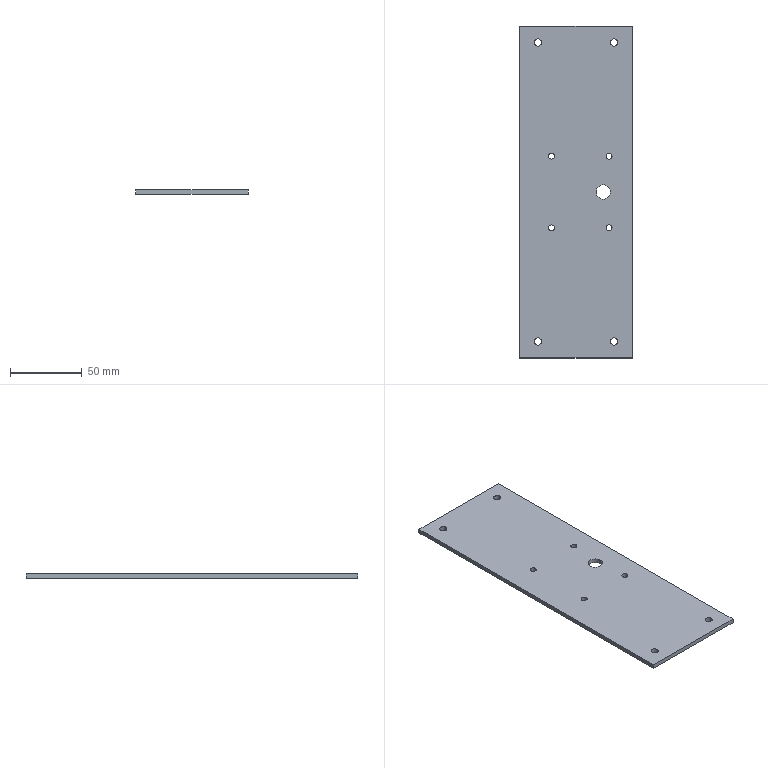Part | SolidWorks | features BaseBody 1 | 1 solid | 24 faces | box 78 x 231 x 3 mm | volume 53417 mm3 | cylinder 18 | plane 6 | commonest cylinder face diameters 4.2 x8 5 x8 10 x2
STEP:
#1=CARTESIAN_POINT('',(-19.1,-25.,3.));
#2=VERTEX_POINT('',#1);
#3=CARTESIAN_POINT('',(-14.9,-25.,3.));
#4=VERTEX_POINT('',#3);
#5=CARTESIAN_POINT('',(-17.,-25.,3.));
#6=DIRECTION('',(0.,0.,1.));
#7=DIRECTION('',(-1.,0.,0.));
#8=AXIS2_PLACEMENT_3D('',#5,#6,#7);
#9=CIRCLE('',#8,2.1);
#10=EDGE_CURVE('',#2,#4,#9,.T.);
#11=ORIENTED_EDGE('',*,*,#10,.T.);
#12=CARTESIAN_POINT('',(-14.9,-25.,0.));
#13=VERTEX_POINT('',#12);
#14=CARTESIAN_POINT('',(-14.9,-25.,3.));
#15=DIRECTION('',(0.,0.,-1.));
#16=VECTOR('',#15,1000.);
#17=LINE('',#14,#16);
#18=EDGE_CURVE('',#4,#13,#17,.T.);
#19=ORIENTED_EDGE('',*,*,#18,.T.);
#20=CARTESIAN_POINT('',(-19.1,-25.,0.));
#21=VERTEX_POINT('',#20);
#22=CARTESIAN_POINT('',(-17.,-25.,0.));
#23=DIRECTION('',(0.,0.,1.));
#24=DIRECTION('',(-1.,0.,0.));
#25=AXIS2_PLACEMENT_3D('',#22,#23,#24);
#26=CIRCLE('',#25,2.1);
#27=EDGE_CURVE('',#21,#13,#26,.T.);
#28=ORIENTED_EDGE('',*,*,#27,.F.);
#29=CARTESIAN_POINT('',(-19.1,-25.,3.));
#30=DIRECTION('',(0.,0.,-1.));
#31=VECTOR('',#30,1000.);
#32=LINE('',#29,#31);
#33=EDGE_CURVE('',#2,#21,#32,.T.);
#34=ORIENTED_EDGE('',*,*,#33,.F.);
#35=EDGE_LOOP('',(#11,#19,#28,#34));
#36=FACE_OUTER_BOUND('',#35,.T.);
#37=CARTESIAN_POINT('',(-17.,-25.,3.));
#38=DIRECTION('',(0.,0.,-1.));
#39=DIRECTION('',(-1.,0.,0.));
#40=AXIS2_PLACEMENT_3D('',#37,#38,#39);
#41=CYLINDRICAL_SURFACE('',#40,2.1);
#42=ADVANCED_FACE('',(#36),#41,.F.);
#43=CARTESIAN_POINT('',(20.9,-25.,3.));
#44=VERTEX_POINT('',#43);
#45=CARTESIAN_POINT('',(25.1,-25.,3.));
#46=VERTEX_POINT('',#45);
#47=CARTESIAN_POINT('',(23.,-25.,3.));
#48=DIRECTION('',(0.,0.,1.));
#49=DIRECTION('',(-1.,0.,0.));
#50=AXIS2_PLACEMENT_3D('',#47,#48,#49);
#51=CIRCLE('',#50,2.1);
#52=EDGE_CURVE('',#44,#46,#51,.T.);
#53=ORIENTED_EDGE('',*,*,#52,.T.);
#54=CARTESIAN_POINT('',(25.1,-25.,0.));
#55=VERTEX_POINT('',#54);
#56=CARTESIAN_POINT('',(25.1,-25.,3.));
#57=DIRECTION('',(0.,0.,-1.));
#58=VECTOR('',#57,1000.);
#59=LINE('',#56,#58);
#60=EDGE_CURVE('',#46,#55,#59,.T.);
#61=ORIENTED_EDGE('',*,*,#60,.T.);
#62=CARTESIAN_POINT('',(20.9,-25.,0.));
#63=VERTEX_POINT('',#62);
#64=CARTESIAN_POINT('',(23.,-25.,0.));
#65=DIRECTION('',(0.,0.,1.));
#66=DIRECTION('',(-1.,0.,0.));
#67=AXIS2_PLACEMENT_3D('',#64,#65,#66);
#68=CIRCLE('',#67,2.1);
#69=EDGE_CURVE('',#63,#55,#68,.T.);
#70=ORIENTED_EDGE('',*,*,#69,.F.);
#71=CARTESIAN_POINT('',(20.9,-25.,3.));
#72=DIRECTION('',(0.,0.,-1.));
#73=VECTOR('',#72,1000.);
#74=LINE('',#71,#73);
#75=EDGE_CURVE('',#44,#63,#74,.T.);
#76=ORIENTED_EDGE('',*,*,#75,.F.);
#77=EDGE_LOOP('',(#53,#61,#70,#76));
#78=FACE_OUTER_BOUND('',#77,.T.);
#79=CARTESIAN_POINT('',(23.,-25.,3.));
#80=DIRECTION('',(0.,0.,-1.));
#81=DIRECTION('',(-1.,0.,0.));
#82=AXIS2_PLACEMENT_3D('',#79,#80,#81);
#83=CYLINDRICAL_SURFACE('',#82,2.1);
#84=ADVANCED_FACE('',(#78),#83,.F.);
#85=CARTESIAN_POINT('',(20.9,25.,3.));
#86=VERTEX_POINT('',#85);
#87=CARTESIAN_POINT('',(25.1,25.,3.));
#88=VERTEX_POINT('',#87);
#89=CARTESIAN_POINT('',(23.,25.,3.));
#90=DIRECTION('',(0.,0.,1.));
#91=DIRECTION('',(-1.,0.,0.));
#92=AXIS2_PLACEMENT_3D('',#89,#90,#91);
#93=CIRCLE('',#92,2.1);
#94=EDGE_CURVE('',#86,#88,#93,.T.);
#95=ORIENTED_EDGE('',*,*,#94,.T.);
#96=CARTESIAN_POINT('',(25.1,25.,0.));
#97=VERTEX_POINT('',#96);
#98=CARTESIAN_POINT('',(25.1,25.,3.));
#99=DIRECTION('',(0.,0.,-1.));
#100=VECTOR('',#99,1000.);
#101=LINE('',#98,#100);
#102=EDGE_CURVE('',#88,#97,#101,.T.);
#103=ORIENTED_EDGE('',*,*,#102,.T.);
#104=CARTESIAN_POINT('',(20.9,25.,0.));
#105=VERTEX_POINT('',#104);
#106=CARTESIAN_POINT('',(23.,25.,0.));
#107=DIRECTION('',(0.,0.,1.));
#108=DIRECTION('',(-1.,0.,0.));
#109=AXIS2_PLACEMENT_3D('',#106,#107,#108);
#110=CIRCLE('',#109,2.1);
#111=EDGE_CURVE('',#105,#97,#110,.T.);
#112=ORIENTED_EDGE('',*,*,#111,.F.);
#113=CARTESIAN_POINT('',(20.9,25.,3.));
#114=DIRECTION('',(0.,0.,-1.));
#115=VECTOR('',#114,1000.);
#116=LINE('',#113,#115);
#117=EDGE_CURVE('',#86,#105,#116,.T.);
#118=ORIENTED_EDGE('',*,*,#117,.F.);
#119=EDGE_LOOP('',(#95,#103,#112,#118));
#120=FACE_OUTER_BOUND('',#119,.T.);
#121=CARTESIAN_POINT('',(23.,25.,3.));
#122=DIRECTION('',(0.,0.,-1.));
#123=DIRECTION('',(-1.,0.,0.));
#124=AXIS2_PLACEMENT_3D('',#121,#122,#123);
#125=CYLINDRICAL_SURFACE('',#124,2.1);
#126=ADVANCED_FACE('',(#120),#125,.F.);
#127=CARTESIAN_POINT('',(14.,0.,3.));
#128=VERTEX_POINT('',#127);
#129=CARTESIAN_POINT('',(24.,0.,3.));
#130=VERTEX_POINT('',#129);
#131=CARTESIAN_POINT('',(19.,0.,3.));
#132=DIRECTION('',(0.,0.,1.));
#133=DIRECTION('',(-1.,0.,0.));
#134=AXIS2_PLACEMENT_3D('',#131,#132,#133);
#135=CIRCLE('',#134,5.);
#136=EDGE_CURVE('',#128,#130,#135,.T.);
#137=ORIENTED_EDGE('',*,*,#136,.T.);
#138=CARTESIAN_POINT('',(24.,0.,0.));
#139=VERTEX_POINT('',#138);
#140=CARTESIAN_POINT('',(24.,0.,3.));
#141=DIRECTION('',(0.,0.,-1.));
#142=VECTOR('',#141,1000.);
#143=LINE('',#140,#142);
#144=EDGE_CURVE('',#130,#139,#143,.T.);
#145=ORIENTED_EDGE('',*,*,#144,.T.);
#146=CARTESIAN_POINT('',(14.,0.,0.));
#147=VERTEX_POINT('',#146);
#148=CARTESIAN_POINT('',(19.,0.,0.));
#149=DIRECTION('',(0.,0.,1.));
#150=DIRECTION('',(-1.,0.,0.));
#151=AXIS2_PLACEMENT_3D('',#148,#149,#150);
#152=CIRCLE('',#151,5.);
#153=EDGE_CURVE('',#147,#139,#152,.T.);
#154=ORIENTED_EDGE('',*,*,#153,.F.);
#155=CARTESIAN_POINT('',(14.,0.,3.));
#156=DIRECTION('',(0.,0.,-1.));
#157=VECTOR('',#156,1000.);
#158=LINE('',#155,#157);
#159=EDGE_CURVE('',#128,#147,#158,.T.);
#160=ORIENTED_EDGE('',*,*,#159,.F.);
#161=EDGE_LOOP('',(#137,#145,#154,#160));
#162=FACE_OUTER_BOUND('',#161,.T.);
#163=CARTESIAN_POINT('',(19.,0.,3.));
#164=DIRECTION('',(0.,0.,-1.));
#165=DIRECTION('',(-1.,0.,0.));
#166=AXIS2_PLACEMENT_3D('',#163,#164,#165);
#167=CYLINDRICAL_SURFACE('',#166,5.);
#168=ADVANCED_FACE('',(#162),#167,.F.);
#169=CARTESIAN_POINT('',(-29.,-104.,3.));
#170=VERTEX_POINT('',#169);
#171=CARTESIAN_POINT('',(-24.,-104.,3.));
#172=VERTEX_POINT('',#171);
#173=CARTESIAN_POINT('',(-26.5,-104.,3.));
#174=DIRECTION('',(0.,0.,1.));
#175=DIRECTION('',(-1.,0.,0.));
#176=AXIS2_PLACEMENT_3D('',#173,#174,#175);
#177=CIRCLE('',#176,2.5);
#178=EDGE_CURVE('',#170,#172,#177,.T.);
#179=ORIENTED_EDGE('',*,*,#178,.T.);
#180=CARTESIAN_POINT('',(-24.,-104.,0.));
#181=VERTEX_POINT('',#180);
#182=CARTESIAN_POINT('',(-24.,-104.,3.));
#183=DIRECTION('',(0.,0.,-1.));
#184=VECTOR('',#183,1000.);
#185=LINE('',#182,#184);
#186=EDGE_CURVE('',#172,#181,#185,.T.);
#187=ORIENTED_EDGE('',*,*,#186,.T.);
#188=CARTESIAN_POINT('',(-29.,-104.,0.));
#189=VERTEX_POINT('',#188);
#190=CARTESIAN_POINT('',(-26.5,-104.,0.));
#191=DIRECTION('',(0.,0.,1.));
#192=DIRECTION('',(-1.,0.,0.));
#193=AXIS2_PLACEMENT_3D('',#190,#191,#192);
#194=CIRCLE('',#193,2.5);
#195=EDGE_CURVE('',#189,#181,#194,.T.);
#196=ORIENTED_EDGE('',*,*,#195,.F.);
#197=CARTESIAN_POINT('',(-29.,-104.,3.));
#198=DIRECTION('',(0.,0.,-1.));
#199=VECTOR('',#198,1000.);
#200=LINE('',#197,#199);
#201=EDGE_CURVE('',#170,#189,#200,.T.);
#202=ORIENTED_EDGE('',*,*,#201,.F.);
#203=EDGE_LOOP('',(#179,#187,#196,#202));
#204=FACE_OUTER_BOUND('',#203,.T.);
#205=CARTESIAN_POINT('',(-26.5,-104.,3.));
#206=DIRECTION('',(0.,0.,-1.));
#207=DIRECTION('',(-1.,0.,0.));
#208=AXIS2_PLACEMENT_3D('',#205,#206,#207);
#209=CYLINDRICAL_SURFACE('',#208,2.5);
#210=ADVANCED_FACE('',(#204),#209,.F.);
#211=CARTESIAN_POINT('',(24.,-104.,3.));
#212=VERTEX_POINT('',#211);
#213=CARTESIAN_POINT('',(29.,-104.,3.));
#214=VERTEX_POINT('',#213);
#215=CARTESIAN_POINT('',(26.5,-104.,3.));
#216=DIRECTION('',(0.,0.,1.));
#217=DIRECTION('',(-1.,0.,0.));
#218=AXIS2_PLACEMENT_3D('',#215,#216,#217);
#219=CIRCLE('',#218,2.5);
#220=EDGE_CURVE('',#212,#214,#219,.T.);
#221=ORIENTED_EDGE('',*,*,#220,.T.);
#222=CARTESIAN_POINT('',(29.,-104.,0.));
#223=VERTEX_POINT('',#222);
#224=CARTESIAN_POINT('',(29.,-104.,3.));
#225=DIRECTION('',(0.,0.,-1.));
#226=VECTOR('',#225,1000.);
#227=LINE('',#224,#226);
#228=EDGE_CURVE('',#214,#223,#227,.T.);
#229=ORIENTED_EDGE('',*,*,#228,.T.);
#230=CARTESIAN_POINT('',(24.,-104.,0.));
#231=VERTEX_POINT('',#230);
#232=CARTESIAN_POINT('',(26.5,-104.,0.));
#233=DIRECTION('',(0.,0.,1.));
#234=DIRECTION('',(-1.,0.,0.));
#235=AXIS2_PLACEMENT_3D('',#232,#233,#234);
#236=CIRCLE('',#235,2.5);
#237=EDGE_CURVE('',#231,#223,#236,.T.);
#238=ORIENTED_EDGE('',*,*,#237,.F.);
#239=CARTESIAN_POINT('',(24.,-104.,3.));
#240=DIRECTION('',(0.,0.,-1.));
#241=VECTOR('',#240,1000.);
#242=LINE('',#239,#241);
#243=EDGE_CURVE('',#212,#231,#242,.T.);
#244=ORIENTED_EDGE('',*,*,#243,.F.);
#245=EDGE_LOOP('',(#221,#229,#238,#244));
#246=FACE_OUTER_BOUND('',#245,.T.);
#247=CARTESIAN_POINT('',(26.5,-104.,3.));
#248=DIRECTION('',(0.,0.,-1.));
#249=DIRECTION('',(-1.,0.,0.));
#250=AXIS2_PLACEMENT_3D('',#247,#248,#249);
#251=CYLINDRICAL_SURFACE('',#250,2.5);
#252=ADVANCED_FACE('',(#246),#251,.F.);
#253=CARTESIAN_POINT('',(24.,104.,3.));
#254=VERTEX_POINT('',#253);
#255=CARTESIAN_POINT('',(29.,104.,3.));
#256=VERTEX_POINT('',#255);
#257=CARTESIAN_POINT('',(26.5,104.,3.));
#258=DIRECTION('',(0.,0.,1.));
#259=DIRECTION('',(-1.,0.,0.));
#260=AXIS2_PLACEMENT_3D('',#257,#258,#259);
#261=CIRCLE('',#260,2.5);
#262=EDGE_CURVE('',#254,#256,#261,.T.);
#263=ORIENTED_EDGE('',*,*,#262,.T.);
#264=CARTESIAN_POINT('',(29.,104.,0.));
#265=VERTEX_POINT('',#264);
#266=CARTESIAN_POINT('',(29.,104.,3.));
#267=DIRECTION('',(0.,0.,-1.));
#268=VECTOR('',#267,1000.);
#269=LINE('',#266,#268);
#270=EDGE_CURVE('',#256,#265,#269,.T.);
#271=ORIENTED_EDGE('',*,*,#270,.T.);
#272=CARTESIAN_POINT('',(24.,104.,0.));
#273=VERTEX_POINT('',#272);
#274=CARTESIAN_POINT('',(26.5,104.,0.));
#275=DIRECTION('',(0.,0.,1.));
#276=DIRECTION('',(-1.,0.,0.));
#277=AXIS2_PLACEMENT_3D('',#274,#275,#276);
#278=CIRCLE('',#277,2.5);
#279=EDGE_CURVE('',#273,#265,#278,.T.);
#280=ORIENTED_EDGE('',*,*,#279,.F.);
#281=CARTESIAN_POINT('',(24.,104.,3.));
#282=DIRECTION('',(0.,0.,-1.));
#283=VECTOR('',#282,1000.);
#284=LINE('',#281,#283);
#285=EDGE_CURVE('',#254,#273,#284,.T.);
#286=ORIENTED_EDGE('',*,*,#285,.F.);
#287=EDGE_LOOP('',(#263,#271,#280,#286));
#288=FACE_OUTER_BOUND('',#287,.T.);
#289=CARTESIAN_POINT('',(26.5,104.,3.));
#290=DIRECTION('',(0.,0.,-1.));
#291=DIRECTION('',(-1.,0.,0.));
#292=AXIS2_PLACEMENT_3D('',#289,#290,#291);
#293=CYLINDRICAL_SURFACE('',#292,2.5);
#294=ADVANCED_FACE('',(#288),#293,.F.);
#295=CARTESIAN_POINT('',(-19.1,25.,3.));
#296=VERTEX_POINT('',#295);
#297=CARTESIAN_POINT('',(-14.9,25.,3.));
#298=VERTEX_POINT('',#297);
#299=CARTESIAN_POINT('',(-17.,25.,3.));
#300=DIRECTION('',(0.,0.,1.));
#301=DIRECTION('',(-1.,0.,0.));
#302=AXIS2_PLACEMENT_3D('',#299,#300,#301);
#303=CIRCLE('',#302,2.1);
#304=EDGE_CURVE('',#296,#298,#303,.T.);
#305=ORIENTED_EDGE('',*,*,#304,.T.);
#306=CARTESIAN_POINT('',(-14.9,25.,0.));
#307=VERTEX_POINT('',#306);
#308=CARTESIAN_POINT('',(-14.9,25.,3.));
#309=DIRECTION('',(0.,0.,-1.));
#310=VECTOR('',#309,1000.);
#311=LINE('',#308,#310);
#312=EDGE_CURVE('',#298,#307,#311,.T.);
#313=ORIENTED_EDGE('',*,*,#312,.T.);
#314=CARTESIAN_POINT('',(-19.1,25.,0.));
#315=VERTEX_POINT('',#314);
#316=CARTESIAN_POINT('',(-17.,25.,0.));
#317=DIRECTION('',(0.,0.,1.));
#318=DIRECTION('',(-1.,0.,0.));
#319=AXIS2_PLACEMENT_3D('',#316,#317,#318);
#320=CIRCLE('',#319,2.1);
#321=EDGE_CURVE('',#315,#307,#320,.T.);
#322=ORIENTED_EDGE('',*,*,#321,.F.);
#323=CARTESIAN_POINT('',(-19.1,25.,3.));
#324=DIRECTION('',(0.,0.,-1.));
#325=VECTOR('',#324,1000.);
#326=LINE('',#323,#325);
#327=EDGE_CURVE('',#296,#315,#326,.T.);
#328=ORIENTED_EDGE('',*,*,#327,.F.);
#329=EDGE_LOOP('',(#305,#313,#322,#328));
#330=FACE_OUTER_BOUND('',#329,.T.);
#331=CARTESIAN_POINT('',(-17.,25.,3.));
#332=DIRECTION('',(0.,0.,-1.));
#333=DIRECTION('',(-1.,0.,0.));
#334=AXIS2_PLACEMENT_3D('',#331,#332,#333);
#335=CYLINDRICAL_SURFACE('',#334,2.1);
#336=ADVANCED_FACE('',(#330),#335,.F.);
#337=CARTESIAN_POINT('',(-29.,104.,3.));
#338=VERTEX_POINT('',#337);
#339=CARTESIAN_POINT('',(-24.,104.,3.));
#340=VERTEX_POINT('',#339);
#341=CARTESIAN_POINT('',(-26.5,104.,3.));
#342=DIRECTION('',(0.,0.,1.));
#343=DIRECTION('',(-1.,0.,0.));
#344=AXIS2_PLACEMENT_3D('',#341,#342,#343);
#345=CIRCLE('',#344,2.5);
#346=EDGE_CURVE('',#338,#340,#345,.T.);
#347=ORIENTED_EDGE('',*,*,#346,.T.);
#348=CARTESIAN_POINT('',(-24.,104.,0.));
#349=VERTEX_POINT('',#348);
#350=CARTESIAN_POINT('',(-24.,104.,3.));
#351=DIRECTION('',(0.,0.,-1.));
#352=VECTOR('',#351,1000.);
#353=LINE('',#350,#352);
#354=EDGE_CURVE('',#340,#349,#353,.T.);
#355=ORIENTED_EDGE('',*,*,#354,.T.);
#356=CARTESIAN_POINT('',(-29.,104.,0.));
#357=VERTEX_POINT('',#356);
#358=CARTESIAN_POINT('',(-26.5,104.,0.));
#359=DIRECTION('',(0.,0.,1.));
#360=DIRECTION('',(-1.,0.,0.));
#361=AXIS2_PLACEMENT_3D('',#358,#359,#360);
#362=CIRCLE('',#361,2.5);
#363=EDGE_CURVE('',#357,#349,#362,.T.);
#364=ORIENTED_EDGE('',*,*,#363,.F.);
#365=CARTESIAN_POINT('',(-29.,104.,3.));
#366=DIRECTION('',(0.,0.,-1.));
#367=VECTOR('',#366,1000.);
#368=LINE('',#365,#367);
#369=EDGE_CURVE('',#338,#357,#368,.T.);
#370=ORIENTED_EDGE('',*,*,#369,.F.);
#371=EDGE_LOOP('',(#347,#355,#364,#370));
#372=FACE_OUTER_BOUND('',#371,.T.);
#373=CARTESIAN_POINT('',(-26.5,104.,3.));
#374=DIRECTION('',(0.,0.,-1.));
#375=DIRECTION('',(-1.,0.,0.));
#376=AXIS2_PLACEMENT_3D('',#373,#374,#375);
#377=CYLINDRICAL_SURFACE('',#376,2.5);
#378=ADVANCED_FACE('',(#372),#377,.F.);
#379=ORIENTED_EDGE('',*,*,#10,.F.);
#380=CARTESIAN_POINT('',(-17.,-25.,3.));
#381=DIRECTION('',(0.,0.,1.));
#382=DIRECTION('',(-1.,0.,0.));
#383=AXIS2_PLACEMENT_3D('',#380,#381,#382);
#384=CIRCLE('',#383,2.1);
#385=EDGE_CURVE('',#4,#2,#384,.T.);
#386=ORIENTED_EDGE('',*,*,#385,.F.);
#387=EDGE_LOOP('',(#379,#386));
#388=FACE_BOUND('',#387,.T.);
#389=ORIENTED_EDGE('',*,*,#52,.F.);
#390=CARTESIAN_POINT('',(23.,-25.,3.));
#391=DIRECTION('',(0.,0.,1.));
#392=DIRECTION('',(-1.,0.,0.));
#393=AXIS2_PLACEMENT_3D('',#390,#391,#392);
#394=CIRCLE('',#393,2.1);
#395=EDGE_CURVE('',#46,#44,#394,.T.);
#396=ORIENTED_EDGE('',*,*,#395,.F.);
#397=EDGE_LOOP('',(#389,#396));
#398=FACE_BOUND('',#397,.T.);
#399=ORIENTED_EDGE('',*,*,#94,.F.);
#400=CARTESIAN_POINT('',(23.,25.,3.));
#401=DIRECTION('',(0.,0.,1.));
#402=DIRECTION('',(-1.,0.,0.));
#403=AXIS2_PLACEMENT_3D('',#400,#401,#402);
#404=CIRCLE('',#403,2.1);
#405=EDGE_CURVE('',#88,#86,#404,.T.);
#406=ORIENTED_EDGE('',*,*,#405,.F.);
#407=EDGE_LOOP('',(#399,#406));
#408=FACE_BOUND('',#407,.T.);
#409=ORIENTED_EDGE('',*,*,#136,.F.);
#410=CARTESIAN_POINT('',(19.,0.,3.));
#411=DIRECTION('',(0.,0.,1.));
#412=DIRECTION('',(-1.,0.,0.));
#413=AXIS2_PLACEMENT_3D('',#410,#411,#412);
#414=CIRCLE('',#413,5.);
#415=EDGE_CURVE('',#130,#128,#414,.T.);
#416=ORIENTED_EDGE('',*,*,#415,.F.);
#417=EDGE_LOOP('',(#409,#416));
#418=FACE_BOUND('',#417,.T.);
#419=ORIENTED_EDGE('',*,*,#178,.F.);
#420=CARTESIAN_POINT('',(-26.5,-104.,3.));
#421=DIRECTION('',(0.,0.,1.));
#422=DIRECTION('',(-1.,0.,0.));
#423=AXIS2_PLACEMENT_3D('',#420,#421,#422);
#424=CIRCLE('',#423,2.5);
#425=EDGE_CURVE('',#172,#170,#424,.T.);
#426=ORIENTED_EDGE('',*,*,#425,.F.);
#427=EDGE_LOOP('',(#419,#426));
#428=FACE_BOUND('',#427,.T.);
#429=ORIENTED_EDGE('',*,*,#220,.F.);
#430=CARTESIAN_POINT('',(26.5,-104.,3.));
#431=DIRECTION('',(0.,0.,1.));
#432=DIRECTION('',(-1.,0.,0.));
#433=AXIS2_PLACEMENT_3D('',#430,#431,#432);
#434=CIRCLE('',#433,2.5);
#435=EDGE_CURVE('',#214,#212,#434,.T.);
#436=ORIENTED_EDGE('',*,*,#435,.F.);
#437=EDGE_LOOP('',(#429,#436));
#438=FACE_BOUND('',#437,.T.);
#439=ORIENTED_EDGE('',*,*,#262,.F.);
#440=CARTESIAN_POINT('',(26.5,104.,3.));
#441=DIRECTION('',(0.,0.,1.));
#442=DIRECTION('',(-1.,0.,0.));
#443=AXIS2_PLACEMENT_3D('',#440,#441,#442);
#444=CIRCLE('',#443,2.5);
#445=EDGE_CURVE('',#256,#254,#444,.T.);
#446=ORIENTED_EDGE('',*,*,#445,.F.);
#447=EDGE_LOOP('',(#439,#446));
#448=FACE_BOUND('',#447,.T.);
#449=ORIENTED_EDGE('',*,*,#304,.F.);
#450=CARTESIAN_POINT('',(-17.,25.,3.));
#451=DIRECTION('',(0.,0.,1.));
#452=DIRECTION('',(-1.,0.,0.));
#453=AXIS2_PLACEMENT_3D('',#450,#451,#452);
#454=CIRCLE('',#453,2.1);
#455=EDGE_CURVE('',#298,#296,#454,.T.);
#456=ORIENTED_EDGE('',*,*,#455,.F.);
#457=EDGE_LOOP('',(#449,#456));
#458=FACE_BOUND('',#457,.T.);
#459=ORIENTED_EDGE('',*,*,#346,.F.);
#460=CARTESIAN_POINT('',(-26.5,104.,3.));
#461=DIRECTION('',(0.,0.,1.));
#462=DIRECTION('',(-1.,0.,0.));
#463=AXIS2_PLACEMENT_3D('',#460,#461,#462);
#464=CIRCLE('',#463,2.5);
#465=EDGE_CURVE('',#340,#338,#464,.T.);
#466=ORIENTED_EDGE('',*,*,#465,.F.);
#467=EDGE_LOOP('',(#459,#466));
#468=FACE_BOUND('',#467,.T.);
#469=CARTESIAN_POINT('',(39.,-115.5,3.));
#470=VERTEX_POINT('',#469);
#471=CARTESIAN_POINT('',(-39.,-115.5,3.));
#472=VERTEX_POINT('',#471);
#473=CARTESIAN_POINT('',(0.,-115.5,3.));
#474=DIRECTION('',(-1.,0.,0.));
#475=VECTOR('',#474,1000.);
#476=LINE('',#473,#475);
#477=EDGE_CURVE('',#470,#472,#476,.T.);
#478=ORIENTED_EDGE('',*,*,#477,.F.);
#479=CARTESIAN_POINT('',(39.,115.5,3.));
#480=VERTEX_POINT('',#479);
#481=CARTESIAN_POINT('',(39.,0.,3.));
#482=DIRECTION('',(0.,-1.,0.));
#483=VECTOR('',#482,1000.);
#484=LINE('',#481,#483);
#485=EDGE_CURVE('',#480,#470,#484,.T.);
#486=ORIENTED_EDGE('',*,*,#485,.F.);
#487=CARTESIAN_POINT('',(-39.,115.5,3.));
#488=VERTEX_POINT('',#487);
#489=CARTESIAN_POINT('',(0.,115.5,3.));
#490=DIRECTION('',(1.,0.,0.));
#491=VECTOR('',#490,1000.);
#492=LINE('',#489,#491);
#493=EDGE_CURVE('',#488,#480,#492,.T.);
#494=ORIENTED_EDGE('',*,*,#493,.F.);
#495=CARTESIAN_POINT('',(-39.,0.,3.));
#496=DIRECTION('',(0.,1.,0.));
#497=VECTOR('',#496,1000.);
#498=LINE('',#495,#497);
#499=EDGE_CURVE('',#472,#488,#498,.T.);
#500=ORIENTED_EDGE('',*,*,#499,.F.);
#501=EDGE_LOOP('',(#478,#486,#494,#500));
#502=FACE_OUTER_BOUND('',#501,.T.);
#503=CARTESIAN_POINT('',(0.,0.,3.));
#504=DIRECTION('',(0.,0.,-1.));
#505=DIRECTION('',(-1.,0.,0.));
#506=AXIS2_PLACEMENT_3D('',#503,#504,#505);
#507=PLANE('',#506);
#508=ADVANCED_FACE('',(#388,#398,#408,#418,#428,#438,#448,#458,#468,#502),#507,.F.);
#509=ORIENTED_EDGE('',*,*,#18,.F.);
#510=ORIENTED_EDGE('',*,*,#385,.T.);
#511=ORIENTED_EDGE('',*,*,#33,.T.);
#512=CARTESIAN_POINT('',(-17.,-25.,0.));
#513=DIRECTION('',(0.,0.,1.));
#514=DIRECTION('',(-1.,0.,0.));
#515=AXIS2_PLACEMENT_3D('',#512,#513,#514);
#516=CIRCLE('',#515,2.1);
#517=EDGE_CURVE('',#13,#21,#516,.T.);
#518=ORIENTED_EDGE('',*,*,#517,.F.);
#519=EDGE_LOOP('',(#509,#510,#511,#518));
#520=FACE_OUTER_BOUND('',#519,.T.);
#521=CARTESIAN_POINT('',(-17.,-25.,3.));
#522=DIRECTION('',(0.,0.,-1.));
#523=DIRECTION('',(-1.,0.,0.));
#524=AXIS2_PLACEMENT_3D('',#521,#522,#523);
#525=CYLINDRICAL_SURFACE('',#524,2.1);
#526=ADVANCED_FACE('',(#520),#525,.F.);
#527=ORIENTED_EDGE('',*,*,#60,.F.);
#528=ORIENTED_EDGE('',*,*,#395,.T.);
#529=ORIENTED_EDGE('',*,*,#75,.T.);
#530=CARTESIAN_POINT('',(23.,-25.,0.));
#531=DIRECTION('',(0.,0.,1.));
#532=DIRECTION('',(-1.,0.,0.));
#533=AXIS2_PLACEMENT_3D('',#530,#531,#532);
#534=CIRCLE('',#533,2.1);
#535=EDGE_CURVE('',#55,#63,#534,.T.);
#536=ORIENTED_EDGE('',*,*,#535,.F.);
#537=EDGE_LOOP('',(#527,#528,#529,#536));
#538=FACE_OUTER_BOUND('',#537,.T.);
#539=CARTESIAN_POINT('',(23.,-25.,3.));
#540=DIRECTION('',(0.,0.,-1.));
#541=DIRECTION('',(-1.,0.,0.));
#542=AXIS2_PLACEMENT_3D('',#539,#540,#541);
#543=CYLINDRICAL_SURFACE('',#542,2.1);
#544=ADVANCED_FACE('',(#538),#543,.F.);
#545=ORIENTED_EDGE('',*,*,#102,.F.);
#546=ORIENTED_EDGE('',*,*,#405,.T.);
#547=ORIENTED_EDGE('',*,*,#117,.T.);
#548=CARTESIAN_POINT('',(23.,25.,0.));
#549=DIRECTION('',(0.,0.,1.));
#550=DIRECTION('',(-1.,0.,0.));
#551=AXIS2_PLACEMENT_3D('',#548,#549,#550);
#552=CIRCLE('',#551,2.1);
#553=EDGE_CURVE('',#97,#105,#552,.T.);
#554=ORIENTED_EDGE('',*,*,#553,.F.);
#555=EDGE_LOOP('',(#545,#546,#547,#554));
#556=FACE_OUTER_BOUND('',#555,.T.);
#557=CARTESIAN_POINT('',(23.,25.,3.));
#558=DIRECTION('',(0.,0.,-1.));
#559=DIRECTION('',(-1.,0.,0.));
#560=AXIS2_PLACEMENT_3D('',#557,#558,#559);
#561=CYLINDRICAL_SURFACE('',#560,2.1);
#562=ADVANCED_FACE('',(#556),#561,.F.);
#563=ORIENTED_EDGE('',*,*,#144,.F.);
#564=ORIENTED_EDGE('',*,*,#415,.T.);
#565=ORIENTED_EDGE('',*,*,#159,.T.);
#566=CARTESIAN_POINT('',(19.,0.,0.));
#567=DIRECTION('',(0.,0.,1.));
#568=DIRECTION('',(-1.,0.,0.));
#569=AXIS2_PLACEMENT_3D('',#566,#567,#568);
#570=CIRCLE('',#569,5.);
#571=EDGE_CURVE('',#139,#147,#570,.T.);
#572=ORIENTED_EDGE('',*,*,#571,.F.);
#573=EDGE_LOOP('',(#563,#564,#565,#572));
#574=FACE_OUTER_BOUND('',#573,.T.);
#575=CARTESIAN_POINT('',(19.,0.,3.));
#576=DIRECTION('',(0.,0.,-1.));
#577=DIRECTION('',(-1.,0.,0.));
#578=AXIS2_PLACEMENT_3D('',#575,#576,#577);
#579=CYLINDRICAL_SURFACE('',#578,5.);
#580=ADVANCED_FACE('',(#574),#579,.F.);
#581=ORIENTED_EDGE('',*,*,#186,.F.);
#582=ORIENTED_EDGE('',*,*,#425,.T.);
#583=ORIENTED_EDGE('',*,*,#201,.T.);
#584=CARTESIAN_POINT('',(-26.5,-104.,0.));
#585=DIRECTION('',(0.,0.,1.));
#586=DIRECTION('',(-1.,0.,0.));
#587=AXIS2_PLACEMENT_3D('',#584,#585,#586);
#588=CIRCLE('',#587,2.5);
#589=EDGE_CURVE('',#181,#189,#588,.T.);
#590=ORIENTED_EDGE('',*,*,#589,.F.);
#591=EDGE_LOOP('',(#581,#582,#583,#590));
#592=FACE_OUTER_BOUND('',#591,.T.);
#593=CARTESIAN_POINT('',(-26.5,-104.,3.));
#594=DIRECTION('',(0.,0.,-1.));
#595=DIRECTION('',(-1.,0.,0.));
#596=AXIS2_PLACEMENT_3D('',#593,#594,#595);
#597=CYLINDRICAL_SURFACE('',#596,2.5);
#598=ADVANCED_FACE('',(#592),#597,.F.);
#599=ORIENTED_EDGE('',*,*,#228,.F.);
#600=ORIENTED_EDGE('',*,*,#435,.T.);
#601=ORIENTED_EDGE('',*,*,#243,.T.);
#602=CARTESIAN_POINT('',(26.5,-104.,0.));
#603=DIRECTION('',(0.,0.,1.));
#604=DIRECTION('',(-1.,0.,0.));
#605=AXIS2_PLACEMENT_3D('',#602,#603,#604);
#606=CIRCLE('',#605,2.5);
#607=EDGE_CURVE('',#223,#231,#606,.T.);
#608=ORIENTED_EDGE('',*,*,#607,.F.);
#609=EDGE_LOOP('',(#599,#600,#601,#608));
#610=FACE_OUTER_BOUND('',#609,.T.);
#611=CARTESIAN_POINT('',(26.5,-104.,3.));
#612=DIRECTION('',(0.,0.,-1.));
#613=DIRECTION('',(-1.,0.,0.));
#614=AXIS2_PLACEMENT_3D('',#611,#612,#613);
#615=CYLINDRICAL_SURFACE('',#614,2.5);
#616=ADVANCED_FACE('',(#610),#615,.F.);
#617=ORIENTED_EDGE('',*,*,#270,.F.);
#618=ORIENTED_EDGE('',*,*,#445,.T.);
#619=ORIENTED_EDGE('',*,*,#285,.T.);
#620=CARTESIAN_POINT('',(26.5,104.,0.));
#621=DIRECTION('',(0.,0.,1.));
#622=DIRECTION('',(-1.,0.,0.));
#623=AXIS2_PLACEMENT_3D('',#620,#621,#622);
#624=CIRCLE('',#623,2.5);
#625=EDGE_CURVE('',#265,#273,#624,.T.);
#626=ORIENTED_EDGE('',*,*,#625,.F.);
#627=EDGE_LOOP('',(#617,#618,#619,#626));
#628=FACE_OUTER_BOUND('',#627,.T.);
#629=CARTESIAN_POINT('',(26.5,104.,3.));
#630=DIRECTION('',(0.,0.,-1.));
#631=DIRECTION('',(-1.,0.,0.));
#632=AXIS2_PLACEMENT_3D('',#629,#630,#631);
#633=CYLINDRICAL_SURFACE('',#632,2.5);
#634=ADVANCED_FACE('',(#628),#633,.F.);
#635=ORIENTED_EDGE('',*,*,#312,.F.);
#636=ORIENTED_EDGE('',*,*,#455,.T.);
#637=ORIENTED_EDGE('',*,*,#327,.T.);
#638=CARTESIAN_POINT('',(-17.,25.,0.));
#639=DIRECTION('',(0.,0.,1.));
#640=DIRECTION('',(-1.,0.,0.));
#641=AXIS2_PLACEMENT_3D('',#638,#639,#640);
#642=CIRCLE('',#641,2.1);
#643=EDGE_CURVE('',#307,#315,#642,.T.);
#644=ORIENTED_EDGE('',*,*,#643,.F.);
#645=EDGE_LOOP('',(#635,#636,#637,#644));
#646=FACE_OUTER_BOUND('',#645,.T.);
#647=CARTESIAN_POINT('',(-17.,25.,3.));
#648=DIRECTION('',(0.,0.,-1.));
#649=DIRECTION('',(-1.,0.,0.));
#650=AXIS2_PLACEMENT_3D('',#647,#648,#649);
#651=CYLINDRICAL_SURFACE('',#650,2.1);
#652=ADVANCED_FACE('',(#646),#651,.F.);
#653=ORIENTED_EDGE('',*,*,#354,.F.);
#654=ORIENTED_EDGE('',*,*,#465,.T.);
#655=ORIENTED_EDGE('',*,*,#369,.T.);
#656=CARTESIAN_POINT('',(-26.5,104.,0.));
#657=DIRECTION('',(0.,0.,1.));
#658=DIRECTION('',(-1.,0.,0.));
#659=AXIS2_PLACEMENT_3D('',#656,#657,#658);
#660=CIRCLE('',#659,2.5);
#661=EDGE_CURVE('',#349,#357,#660,.T.);
#662=ORIENTED_EDGE('',*,*,#661,.F.);
#663=EDGE_LOOP('',(#653,#654,#655,#662));
#664=FACE_OUTER_BOUND('',#663,.T.);
#665=CARTESIAN_POINT('',(-26.5,104.,3.));
#666=DIRECTION('',(0.,0.,-1.));
#667=DIRECTION('',(-1.,0.,0.));
#668=AXIS2_PLACEMENT_3D('',#665,#666,#667);
#669=CYLINDRICAL_SURFACE('',#668,2.5);
#670=ADVANCED_FACE('',(#664),#669,.F.);
#671=CARTESIAN_POINT('',(-39.,-115.5,0.));
#672=VERTEX_POINT('',#671);
#673=CARTESIAN_POINT('',(-39.,-115.5,3.));
#674=DIRECTION('',(0.,0.,-1.));
#675=VECTOR('',#674,1000.);
#676=LINE('',#673,#675);
#677=EDGE_CURVE('',#472,#672,#676,.T.);
#678=ORIENTED_EDGE('',*,*,#677,.F.);
#679=ORIENTED_EDGE('',*,*,#499,.T.);
#680=CARTESIAN_POINT('',(-39.,115.5,0.));
#681=VERTEX_POINT('',#680);
#682=CARTESIAN_POINT('',(-39.,115.5,3.));
#683=DIRECTION('',(0.,0.,1.));
#684=VECTOR('',#683,1000.);
#685=LINE('',#682,#684);
#686=EDGE_CURVE('',#681,#488,#685,.T.);
#687=ORIENTED_EDGE('',*,*,#686,.F.);
#688=CARTESIAN_POINT('',(-39.,115.5,0.));
#689=DIRECTION('',(0.,1.,0.));
#690=VECTOR('',#689,1000.);
#691=LINE('',#688,#690);
#692=EDGE_CURVE('',#672,#681,#691,.T.);
#693=ORIENTED_EDGE('',*,*,#692,.F.);
#694=EDGE_LOOP('',(#678,#679,#687,#693));
#695=FACE_OUTER_BOUND('',#694,.T.);
#696=CARTESIAN_POINT('',(-39.,115.5,3.));
#697=DIRECTION('',(1.,0.,0.));
#698=DIRECTION('',(0.,1.,0.));
#699=AXIS2_PLACEMENT_3D('',#696,#697,#698);
#700=PLANE('',#699);
#701=ADVANCED_FACE('',(#695),#700,.F.);
#702=CARTESIAN_POINT('',(39.,-115.5,0.));
#703=VERTEX_POINT('',#702);
#704=CARTESIAN_POINT('',(39.,-115.5,3.));
#705=DIRECTION('',(0.,0.,-1.));
#706=VECTOR('',#705,1000.);
#707=LINE('',#704,#706);
#708=EDGE_CURVE('',#470,#703,#707,.T.);
#709=ORIENTED_EDGE('',*,*,#708,.F.);
#710=ORIENTED_EDGE('',*,*,#477,.T.);
#711=ORIENTED_EDGE('',*,*,#677,.T.);
#712=CARTESIAN_POINT('',(39.,-115.5,0.));
#713=DIRECTION('',(-1.,0.,0.));
#714=VECTOR('',#713,1000.);
#715=LINE('',#712,#714);
#716=EDGE_CURVE('',#703,#672,#715,.T.);
#717=ORIENTED_EDGE('',*,*,#716,.F.);
#718=EDGE_LOOP('',(#709,#710,#711,#717));
#719=FACE_OUTER_BOUND('',#718,.T.);
#720=CARTESIAN_POINT('',(39.,-115.5,3.));
#721=DIRECTION('',(0.,1.,0.));
#722=DIRECTION('',(-1.,0.,0.));
#723=AXIS2_PLACEMENT_3D('',#720,#721,#722);
#724=PLANE('',#723);
#725=ADVANCED_FACE('',(#719),#724,.F.);
#726=CARTESIAN_POINT('',(39.,115.5,0.));
#727=VERTEX_POINT('',#726);
#728=CARTESIAN_POINT('',(39.,115.5,3.));
#729=DIRECTION('',(0.,0.,-1.));
#730=VECTOR('',#729,1000.);
#731=LINE('',#728,#730);
#732=EDGE_CURVE('',#480,#727,#731,.T.);
#733=ORIENTED_EDGE('',*,*,#732,.F.);
#734=ORIENTED_EDGE('',*,*,#485,.T.);
#735=ORIENTED_EDGE('',*,*,#708,.T.);
#736=CARTESIAN_POINT('',(39.,115.5,0.));
#737=DIRECTION('',(0.,-1.,0.));
#738=VECTOR('',#737,1000.);
#739=LINE('',#736,#738);
#740=EDGE_CURVE('',#727,#703,#739,.T.);
#741=ORIENTED_EDGE('',*,*,#740,.F.);
#742=EDGE_LOOP('',(#733,#734,#735,#741));
#743=FACE_OUTER_BOUND('',#742,.T.);
#744=CARTESIAN_POINT('',(39.,115.5,3.));
#745=DIRECTION('',(-1.,0.,0.));
#746=DIRECTION('',(0.,-1.,0.));
#747=AXIS2_PLACEMENT_3D('',#744,#745,#746);
#748=PLANE('',#747);
#749=ADVANCED_FACE('',(#743),#748,.F.);
#750=ORIENTED_EDGE('',*,*,#686,.T.);
#751=ORIENTED_EDGE('',*,*,#493,.T.);
#752=ORIENTED_EDGE('',*,*,#732,.T.);
#753=CARTESIAN_POINT('',(39.,115.5,0.));
#754=DIRECTION('',(1.,0.,0.));
#755=VECTOR('',#754,1000.);
#756=LINE('',#753,#755);
#757=EDGE_CURVE('',#681,#727,#756,.T.);
#758=ORIENTED_EDGE('',*,*,#757,.F.);
#759=EDGE_LOOP('',(#750,#751,#752,#758));
#760=FACE_OUTER_BOUND('',#759,.T.);
#761=CARTESIAN_POINT('',(39.,115.5,3.));
#762=DIRECTION('',(0.,-1.,0.));
#763=DIRECTION('',(0.,0.,-1.));
#764=AXIS2_PLACEMENT_3D('',#761,#762,#763);
#765=PLANE('',#764);
#766=ADVANCED_FACE('',(#760),#765,.F.);
#767=ORIENTED_EDGE('',*,*,#27,.T.);
#768=ORIENTED_EDGE('',*,*,#517,.T.);
#769=EDGE_LOOP('',(#767,#768));
#770=FACE_BOUND('',#769,.T.);
#771=ORIENTED_EDGE('',*,*,#111,.T.);
#772=ORIENTED_EDGE('',*,*,#553,.T.);
#773=EDGE_LOOP('',(#771,#772));
#774=FACE_BOUND('',#773,.T.);
#775=ORIENTED_EDGE('',*,*,#195,.T.);
#776=ORIENTED_EDGE('',*,*,#589,.T.);
#777=EDGE_LOOP('',(#775,#776));
#778=FACE_BOUND('',#777,.T.);
#779=ORIENTED_EDGE('',*,*,#279,.T.);
#780=ORIENTED_EDGE('',*,*,#625,.T.);
#781=EDGE_LOOP('',(#779,#780));
#782=FACE_BOUND('',#781,.T.);
#783=ORIENTED_EDGE('',*,*,#363,.T.);
#784=ORIENTED_EDGE('',*,*,#661,.T.);
#785=EDGE_LOOP('',(#783,#784));
#786=FACE_BOUND('',#785,.T.);
#787=ORIENTED_EDGE('',*,*,#321,.T.);
#788=ORIENTED_EDGE('',*,*,#643,.T.);
#789=EDGE_LOOP('',(#787,#788));
#790=FACE_BOUND('',#789,.T.);
#791=ORIENTED_EDGE('',*,*,#237,.T.);
#792=ORIENTED_EDGE('',*,*,#607,.T.);
#793=EDGE_LOOP('',(#791,#792));
#794=FACE_BOUND('',#793,.T.);
#795=ORIENTED_EDGE('',*,*,#153,.T.);
#796=ORIENTED_EDGE('',*,*,#571,.T.);
#797=EDGE_LOOP('',(#795,#796));
#798=FACE_BOUND('',#797,.T.);
#799=ORIENTED_EDGE('',*,*,#69,.T.);
#800=ORIENTED_EDGE('',*,*,#535,.T.);
#801=EDGE_LOOP('',(#799,#800));
#802=FACE_BOUND('',#801,.T.);
#803=ORIENTED_EDGE('',*,*,#740,.T.);
#804=ORIENTED_EDGE('',*,*,#716,.T.);
#805=ORIENTED_EDGE('',*,*,#692,.T.);
#806=ORIENTED_EDGE('',*,*,#757,.T.);
#807=EDGE_LOOP('',(#803,#804,#805,#806));
#808=FACE_OUTER_BOUND('',#807,.T.);
#809=CARTESIAN_POINT('',(0.,0.,0.));
#810=DIRECTION('',(0.,0.,-1.));
#811=DIRECTION('',(-1.,0.,0.));
#812=AXIS2_PLACEMENT_3D('',#809,#810,#811);
#813=PLANE('',#812);
#814=ADVANCED_FACE('',(#770,#774,#778,#782,#786,#790,#794,#798,#802,#808),#813,.T.);
#815=CLOSED_SHELL('',(#42,#84,#126,#168,#210,#252,#294,#336,#378,#508,#526,#544,#562,#580,#598,#616,#634,#652,#670,#701,#725,#749,#766,#814));
#816=MANIFOLD_SOLID_BREP('',#815);
#817=CARTESIAN_POINT('',(0.,0.,0.));
#818=DIRECTION('',(0.,0.,1.));
#819=DIRECTION('',(1.,0.,0.));
#820=AXIS2_PLACEMENT_3D('',#817,#818,#819);
#821=(LENGTH_UNIT()NAMED_UNIT(*)SI_UNIT(.MILLI.,.METRE.));
#822=UNCERTAINTY_MEASURE_WITH_UNIT(LENGTH_MEASURE(0.00001),#821,'','');
#823=(NAMED_UNIT(*)PLANE_ANGLE_UNIT()SI_UNIT($,.RADIAN.));
#824=(NAMED_UNIT(*)SI_UNIT($,.STERADIAN.)SOLID_ANGLE_UNIT());
#825=(GEOMETRIC_REPRESENTATION_CONTEXT(3)GLOBAL_UNCERTAINTY_ASSIGNED_CONTEXT((#822))GLOBAL_UNIT_ASSIGNED_CONTEXT((#821,#823,#824))REPRESENTATION_CONTEXT('',''));
#826=ADVANCED_BREP_SHAPE_REPRESENTATION('',(#816,#820),#825);